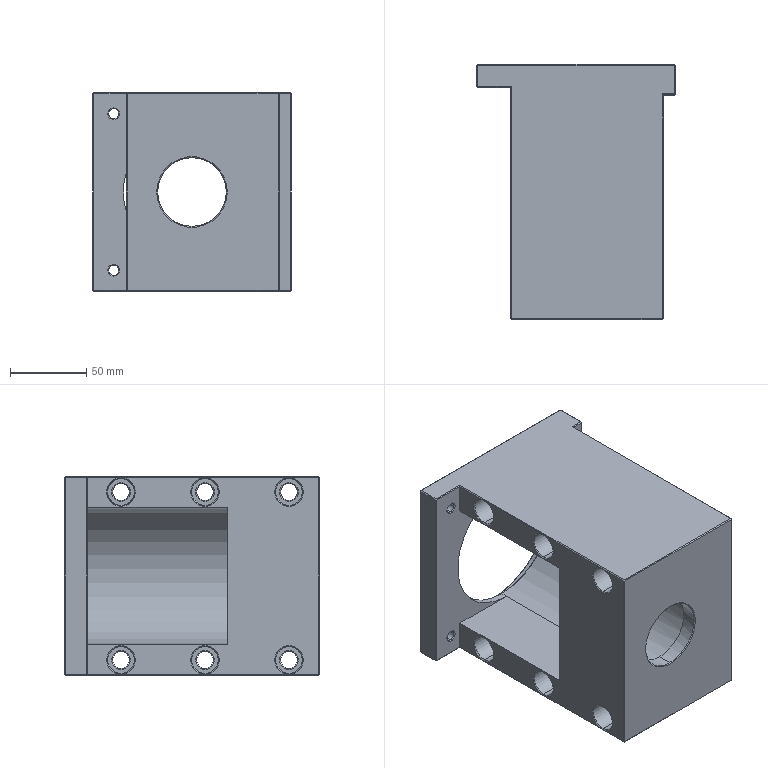Part | SolidWorks | features ICE 2, BaseBody 1, BossThin 1, DelFace 1, DeleteBody 1 | 1 solid | 157 faces | box 130 x 167 x 130 mm | volume 1168663 mm3 | cone 60 | plane 57 | cylinder 40 | commonest cylinder face diameters 11 x12 17.5 x12 6.5 x8 45 x2 62 x2 90 x2